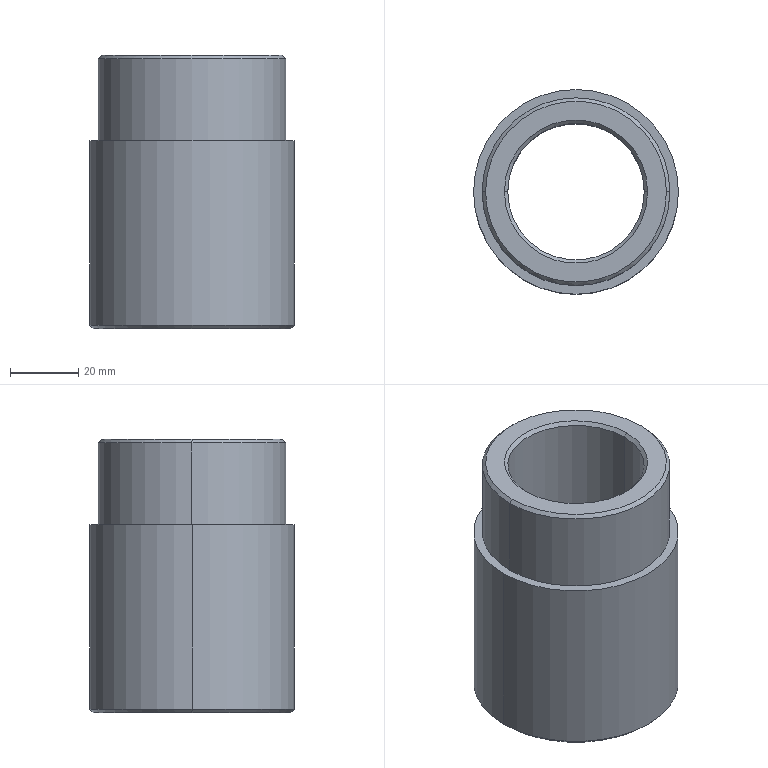Part | STEP file | Bac truot | 1 solid | 17 faces | box 60 x 60 x 80 mm | volume 114067 mm3 | cone 8 | cylinder 6 | plane 3 | commonest cylinder face diameters 40 x2 55 x2 60 x2
STEP:
#1=CARTESIAN_POINT('',(0.,0.,0.));
#2=DIRECTION('',(0.,0.,1.));
#3=DIRECTION('',(1.,0.,0.));
#4=AXIS2_PLACEMENT_3D('',#1,#2,#3);
#5=CARTESIAN_POINT('',(20.,0.,39.));
#6=VERTEX_POINT('',#5);
#7=CARTESIAN_POINT('',(21.,0.,40.));
#8=VERTEX_POINT('',#7);
#9=CARTESIAN_POINT('',(20.,0.,39.));
#10=DIRECTION('',(0.7071,0.,0.7071));
#11=VECTOR('',#10,1.);
#12=LINE('',#9,#11);
#13=CARTESIAN_POINT('',(0.,0.,39.));
#14=DIRECTION('',(0.,0.,1.));
#15=DIRECTION('',(1.,0.,0.));
#16=AXIS2_PLACEMENT_3D('',#13,#14,#15);
#17=CONICAL_SURFACE('',#16,20.,0.7854);
#18=CARTESIAN_POINT('',(6.283,0.));
#19=DIRECTION('',(0.,1.));
#20=VECTOR('',#19,1.);
#21=LINE('',#18,#20);
#22=(GEOMETRIC_REPRESENTATION_CONTEXT(2)PARAMETRIC_REPRESENTATION_CONTEXT()REPRESENTATION_CONTEXT('',''));
#23=DEFINITIONAL_REPRESENTATION('',(#21),#22);
#24=PCURVE('',#17,#23);
#25=CARTESIAN_POINT('',(0.,0.,39.));
#26=DIRECTION('',(0.,0.,1.));
#27=DIRECTION('',(1.,0.,0.));
#28=AXIS2_PLACEMENT_3D('',#25,#26,#27);
#29=CONICAL_SURFACE('',#28,20.,0.7854);
#30=CARTESIAN_POINT('',(0.,0.));
#31=DIRECTION('',(0.,1.));
#32=VECTOR('',#31,1.);
#33=LINE('',#30,#32);
#34=(GEOMETRIC_REPRESENTATION_CONTEXT(2)PARAMETRIC_REPRESENTATION_CONTEXT()REPRESENTATION_CONTEXT('',''));
#35=DEFINITIONAL_REPRESENTATION('',(#33),#34);
#36=PCURVE('',#29,#35);
#37=SURFACE_CURVE('',#12,(#24,#36),.PCURVE_S1.);
#38=EDGE_CURVE('',#6,#8,#37,.T.);
#39=ORIENTED_EDGE('',*,*,#38,.T.);
#40=CARTESIAN_POINT('',(-21.,0.,40.));
#41=VERTEX_POINT('',#40);
#42=CARTESIAN_POINT('',(0.,0.,40.));
#43=DIRECTION('',(0.,0.,-1.));
#44=DIRECTION('',(1.,0.,0.));
#45=AXIS2_PLACEMENT_3D('',#42,#43,#44);
#46=CIRCLE('',#45,21.);
#47=CARTESIAN_POINT('',(6.283,1.));
#48=DIRECTION('',(-1.,0.));
#49=VECTOR('',#48,1.);
#50=LINE('',#47,#49);
#51=(GEOMETRIC_REPRESENTATION_CONTEXT(2)PARAMETRIC_REPRESENTATION_CONTEXT()REPRESENTATION_CONTEXT('',''));
#52=DEFINITIONAL_REPRESENTATION('',(#50),#51);
#53=PCURVE('',#17,#52);
#54=CARTESIAN_POINT('',(0.,0.,40.));
#55=DIRECTION('',(0.,0.,1.));
#56=DIRECTION('',(1.,0.,0.));
#57=AXIS2_PLACEMENT_3D('',#54,#55,#56);
#58=PLANE('',#57);
#59=CARTESIAN_POINT('',(21.,0.));
#60=CARTESIAN_POINT('',(21.,-36.373));
#61=CARTESIAN_POINT('',(-10.5,-18.187));
#62=CARTESIAN_POINT('',(-42.,0.));
#63=CARTESIAN_POINT('',(-10.5,18.187));
#64=CARTESIAN_POINT('',(21.,36.373));
#65=CARTESIAN_POINT('',(21.,0.));
#66=(BOUNDED_CURVE()B_SPLINE_CURVE(2,(#59,#60,#61,#62,#63,#64,#65),.UNSPECIFIED.,.T.,.F.)B_SPLINE_CURVE_WITH_KNOTS((1,2,2,2,2,1),(-2.094,0.,2.094,4.189,6.283,8.378),.UNSPECIFIED.)CURVE()GEOMETRIC_REPRESENTATION_ITEM()RATIONAL_B_SPLINE_CURVE((1.,0.5,1.,0.5,1.,0.5,1.))REPRESENTATION_ITEM(''));
#67=(GEOMETRIC_REPRESENTATION_CONTEXT(2)PARAMETRIC_REPRESENTATION_CONTEXT()REPRESENTATION_CONTEXT('',''));
#68=DEFINITIONAL_REPRESENTATION('',(#66),#67);
#69=PCURVE('',#58,#68);
#70=SURFACE_CURVE('',#46,(#53,#69),.PCURVE_S1.);
#71=EDGE_CURVE('',#8,#41,#70,.T.);
#72=ORIENTED_EDGE('',*,*,#71,.T.);
#73=CARTESIAN_POINT('',(-20.,0.,39.));
#74=VERTEX_POINT('',#73);
#75=CARTESIAN_POINT('',(-20.,0.,39.));
#76=DIRECTION('',(-0.7071,0.,0.7071));
#77=VECTOR('',#76,1.);
#78=LINE('',#75,#77);
#79=CARTESIAN_POINT('',(3.142,0.));
#80=DIRECTION('',(0.,1.));
#81=VECTOR('',#80,1.);
#82=LINE('',#79,#81);
#83=(GEOMETRIC_REPRESENTATION_CONTEXT(2)PARAMETRIC_REPRESENTATION_CONTEXT()REPRESENTATION_CONTEXT('',''));
#84=DEFINITIONAL_REPRESENTATION('',(#82),#83);
#85=PCURVE('',#17,#84);
#86=CARTESIAN_POINT('',(3.142,0.));
#87=DIRECTION('',(0.,1.));
#88=VECTOR('',#87,1.);
#89=LINE('',#86,#88);
#90=(GEOMETRIC_REPRESENTATION_CONTEXT(2)PARAMETRIC_REPRESENTATION_CONTEXT()REPRESENTATION_CONTEXT('',''));
#91=DEFINITIONAL_REPRESENTATION('',(#89),#90);
#92=PCURVE('',#29,#91);
#93=SURFACE_CURVE('',#78,(#85,#92),.PCURVE_S1.);
#94=EDGE_CURVE('',#74,#41,#93,.T.);
#95=ORIENTED_EDGE('',*,*,#94,.F.);
#96=CARTESIAN_POINT('',(0.,0.,39.));
#97=DIRECTION('',(0.,0.,1.));
#98=DIRECTION('',(1.,0.,0.));
#99=AXIS2_PLACEMENT_3D('',#96,#97,#98);
#100=CIRCLE('',#99,20.);
#101=CARTESIAN_POINT('',(0.,0.));
#102=DIRECTION('',(1.,0.));
#103=VECTOR('',#102,1.);
#104=LINE('',#101,#103);
#105=(GEOMETRIC_REPRESENTATION_CONTEXT(2)PARAMETRIC_REPRESENTATION_CONTEXT()REPRESENTATION_CONTEXT('',''));
#106=DEFINITIONAL_REPRESENTATION('',(#104),#105);
#107=PCURVE('',#17,#106);
#108=CARTESIAN_POINT('',(0.,0.,40.));
#109=DIRECTION('',(0.,0.,-1.));
#110=DIRECTION('',(-1.,0.,0.));
#111=AXIS2_PLACEMENT_3D('',#108,#109,#110);
#112=CYLINDRICAL_SURFACE('',#111,20.);
#113=CARTESIAN_POINT('',(9.425,1.));
#114=DIRECTION('',(-1.,0.));
#115=VECTOR('',#114,1.);
#116=LINE('',#113,#115);
#117=(GEOMETRIC_REPRESENTATION_CONTEXT(2)PARAMETRIC_REPRESENTATION_CONTEXT()REPRESENTATION_CONTEXT('',''));
#118=DEFINITIONAL_REPRESENTATION('',(#116),#117);
#119=PCURVE('',#112,#118);
#120=SURFACE_CURVE('',#100,(#107,#119),.PCURVE_S1.);
#121=EDGE_CURVE('',#74,#6,#120,.T.);
#122=ORIENTED_EDGE('',*,*,#121,.T.);
#123=EDGE_LOOP('',(#39,#72,#95,#122));
#124=FACE_BOUND('',#123,.F.);
#125=ADVANCED_FACE('',(#124),#17,.F.);
#126=CARTESIAN_POINT('',(26.5,0.,40.));
#127=VERTEX_POINT('',#126);
#128=CARTESIAN_POINT('',(-26.5,0.,40.));
#129=VERTEX_POINT('',#128);
#130=CARTESIAN_POINT('',(0.,0.,40.));
#131=DIRECTION('',(0.,0.,1.));
#132=DIRECTION('',(1.,0.,0.));
#133=AXIS2_PLACEMENT_3D('',#130,#131,#132);
#134=CIRCLE('',#133,26.5);
#135=CARTESIAN_POINT('',(0.,0.,40.));
#136=DIRECTION('',(0.,0.,-1.));
#137=DIRECTION('',(-1.,0.,0.));
#138=AXIS2_PLACEMENT_3D('',#135,#136,#137);
#139=CONICAL_SURFACE('',#138,26.5,0.7854);
#140=CARTESIAN_POINT('',(3.142,0.));
#141=DIRECTION('',(-1.,0.));
#142=VECTOR('',#141,1.);
#143=LINE('',#140,#142);
#144=(GEOMETRIC_REPRESENTATION_CONTEXT(2)PARAMETRIC_REPRESENTATION_CONTEXT()REPRESENTATION_CONTEXT('',''));
#145=DEFINITIONAL_REPRESENTATION('',(#143),#144);
#146=PCURVE('',#139,#145);
#147=CARTESIAN_POINT('',(0.,0.));
#148=DIRECTION('',(1.,0.));
#149=AXIS2_PLACEMENT_2D('',#147,#148);
#150=CIRCLE('',#149,26.5);
#151=(GEOMETRIC_REPRESENTATION_CONTEXT(2)PARAMETRIC_REPRESENTATION_CONTEXT()REPRESENTATION_CONTEXT('',''));
#152=DEFINITIONAL_REPRESENTATION('',(#150),#151);
#153=PCURVE('',#58,#152);
#154=SURFACE_CURVE('',#134,(#146,#153),.PCURVE_S1.);
#155=EDGE_CURVE('',#127,#129,#154,.T.);
#156=ORIENTED_EDGE('',*,*,#155,.F.);
#157=CARTESIAN_POINT('',(27.5,0.,39.));
#158=VERTEX_POINT('',#157);
#159=CARTESIAN_POINT('',(26.5,0.,40.));
#160=DIRECTION('',(0.7071,0.,-0.7071));
#161=VECTOR('',#160,1.);
#162=LINE('',#159,#161);
#163=CARTESIAN_POINT('',(3.142,0.));
#164=DIRECTION('',(0.,1.));
#165=VECTOR('',#164,1.);
#166=LINE('',#163,#165);
#167=(GEOMETRIC_REPRESENTATION_CONTEXT(2)PARAMETRIC_REPRESENTATION_CONTEXT()REPRESENTATION_CONTEXT('',''));
#168=DEFINITIONAL_REPRESENTATION('',(#166),#167);
#169=PCURVE('',#139,#168);
#170=CARTESIAN_POINT('',(0.,0.,40.));
#171=DIRECTION('',(0.,0.,-1.));
#172=DIRECTION('',(-1.,0.,0.));
#173=AXIS2_PLACEMENT_3D('',#170,#171,#172);
#174=CONICAL_SURFACE('',#173,26.5,0.7854);
#175=CARTESIAN_POINT('',(3.142,0.));
#176=DIRECTION('',(0.,1.));
#177=VECTOR('',#176,1.);
#178=LINE('',#175,#177);
#179=(GEOMETRIC_REPRESENTATION_CONTEXT(2)PARAMETRIC_REPRESENTATION_CONTEXT()REPRESENTATION_CONTEXT('',''));
#180=DEFINITIONAL_REPRESENTATION('',(#178),#179);
#181=PCURVE('',#174,#180);
#182=SURFACE_CURVE('',#162,(#169,#181),.PCURVE_S1.);
#183=EDGE_CURVE('',#127,#158,#182,.T.);
#184=ORIENTED_EDGE('',*,*,#183,.T.);
#185=CARTESIAN_POINT('',(-27.5,0.,39.));
#186=VERTEX_POINT('',#185);
#187=CARTESIAN_POINT('',(0.,0.,39.));
#188=DIRECTION('',(0.,0.,-1.));
#189=DIRECTION('',(1.,0.,0.));
#190=AXIS2_PLACEMENT_3D('',#187,#188,#189);
#191=CIRCLE('',#190,27.5);
#192=CARTESIAN_POINT('',(-3.142,1.));
#193=DIRECTION('',(1.,0.));
#194=VECTOR('',#193,1.);
#195=LINE('',#192,#194);
#196=(GEOMETRIC_REPRESENTATION_CONTEXT(2)PARAMETRIC_REPRESENTATION_CONTEXT()REPRESENTATION_CONTEXT('',''));
#197=DEFINITIONAL_REPRESENTATION('',(#195),#196);
#198=PCURVE('',#139,#197);
#199=CARTESIAN_POINT('',(0.,0.,15.));
#200=DIRECTION('',(0.,0.,1.));
#201=DIRECTION('',(1.,0.,0.));
#202=AXIS2_PLACEMENT_3D('',#199,#200,#201);
#203=CYLINDRICAL_SURFACE('',#202,27.5);
#204=CARTESIAN_POINT('',(6.283,24.));
#205=DIRECTION('',(-1.,0.));
#206=VECTOR('',#205,1.);
#207=LINE('',#204,#206);
#208=(GEOMETRIC_REPRESENTATION_CONTEXT(2)PARAMETRIC_REPRESENTATION_CONTEXT()REPRESENTATION_CONTEXT('',''));
#209=DEFINITIONAL_REPRESENTATION('',(#207),#208);
#210=PCURVE('',#203,#209);
#211=SURFACE_CURVE('',#191,(#198,#210),.PCURVE_S1.);
#212=EDGE_CURVE('',#186,#158,#211,.T.);
#213=ORIENTED_EDGE('',*,*,#212,.F.);
#214=CARTESIAN_POINT('',(-26.5,0.,40.));
#215=DIRECTION('',(-0.7071,0.,-0.7071));
#216=VECTOR('',#215,1.);
#217=LINE('',#214,#216);
#218=CARTESIAN_POINT('',(0.,0.));
#219=DIRECTION('',(0.,1.));
#220=VECTOR('',#219,1.);
#221=LINE('',#218,#220);
#222=(GEOMETRIC_REPRESENTATION_CONTEXT(2)PARAMETRIC_REPRESENTATION_CONTEXT()REPRESENTATION_CONTEXT('',''));
#223=DEFINITIONAL_REPRESENTATION('',(#221),#222);
#224=PCURVE('',#139,#223);
#225=CARTESIAN_POINT('',(6.283,0.));
#226=DIRECTION('',(0.,1.));
#227=VECTOR('',#226,1.);
#228=LINE('',#225,#227);
#229=(GEOMETRIC_REPRESENTATION_CONTEXT(2)PARAMETRIC_REPRESENTATION_CONTEXT()REPRESENTATION_CONTEXT('',''));
#230=DEFINITIONAL_REPRESENTATION('',(#228),#229);
#231=PCURVE('',#174,#230);
#232=SURFACE_CURVE('',#217,(#224,#231),.PCURVE_S1.);
#233=EDGE_CURVE('',#129,#186,#232,.T.);
#234=ORIENTED_EDGE('',*,*,#233,.F.);
#235=EDGE_LOOP('',(#156,#184,#213,#234));
#236=FACE_BOUND('',#235,.T.);
#237=ADVANCED_FACE('',(#236),#139,.T.);
#238=CARTESIAN_POINT('',(-29.,0.,-40.));
#239=VERTEX_POINT('',#238);
#240=CARTESIAN_POINT('',(29.,0.,-40.));
#241=VERTEX_POINT('',#240);
#242=CARTESIAN_POINT('',(0.,0.,-40.));
#243=DIRECTION('',(0.,0.,-1.));
#244=DIRECTION('',(1.,0.,0.));
#245=AXIS2_PLACEMENT_3D('',#242,#243,#244);
#246=CIRCLE('',#245,29.);
#247=CARTESIAN_POINT('',(0.,0.,-39.));
#248=DIRECTION('',(0.,0.,1.));
#249=DIRECTION('',(1.,0.,0.));
#250=AXIS2_PLACEMENT_3D('',#247,#248,#249);
#251=CONICAL_SURFACE('',#250,30.,0.7854);
#252=CARTESIAN_POINT('',(6.283,-1.));
#253=DIRECTION('',(-1.,0.));
#254=VECTOR('',#253,1.);
#255=LINE('',#252,#254);
#256=(GEOMETRIC_REPRESENTATION_CONTEXT(2)PARAMETRIC_REPRESENTATION_CONTEXT()REPRESENTATION_CONTEXT('',''));
#257=DEFINITIONAL_REPRESENTATION('',(#255),#256);
#258=PCURVE('',#251,#257);
#259=CARTESIAN_POINT('',(0.,0.,-40.));
#260=DIRECTION('',(0.,0.,1.));
#261=DIRECTION('',(1.,0.,0.));
#262=AXIS2_PLACEMENT_3D('',#259,#260,#261);
#263=PLANE('',#262);
#264=CARTESIAN_POINT('',(29.,0.));
#265=CARTESIAN_POINT('',(29.,-50.229));
#266=CARTESIAN_POINT('',(-14.5,-25.115));
#267=CARTESIAN_POINT('',(-58.,0.));
#268=CARTESIAN_POINT('',(-14.5,25.115));
#269=CARTESIAN_POINT('',(29.,50.229));
#270=CARTESIAN_POINT('',(29.,0.));
#271=(BOUNDED_CURVE()B_SPLINE_CURVE(2,(#264,#265,#266,#267,#268,#269,#270),.UNSPECIFIED.,.T.,.F.)B_SPLINE_CURVE_WITH_KNOTS((1,2,2,2,2,1),(-2.094,0.,2.094,4.189,6.283,8.378),.UNSPECIFIED.)CURVE()GEOMETRIC_REPRESENTATION_ITEM()RATIONAL_B_SPLINE_CURVE((1.,0.5,1.,0.5,1.,0.5,1.))REPRESENTATION_ITEM(''));
#272=(GEOMETRIC_REPRESENTATION_CONTEXT(2)PARAMETRIC_REPRESENTATION_CONTEXT()REPRESENTATION_CONTEXT('',''));
#273=DEFINITIONAL_REPRESENTATION('',(#271),#272);
#274=PCURVE('',#263,#273);
#275=SURFACE_CURVE('',#246,(#258,#274),.PCURVE_S1.);
#276=EDGE_CURVE('',#239,#241,#275,.T.);
#277=ORIENTED_EDGE('',*,*,#276,.F.);
#278=CARTESIAN_POINT('',(-30.,0.,-39.));
#279=VERTEX_POINT('',#278);
#280=CARTESIAN_POINT('',(-30.,0.,-39.));
#281=DIRECTION('',(-0.7071,0.,0.7071));
#282=VECTOR('',#281,1.);
#283=LINE('',#280,#282);
#284=CARTESIAN_POINT('',(3.142,0.));
#285=DIRECTION('',(0.,1.));
#286=VECTOR('',#285,1.);
#287=LINE('',#284,#286);
#288=(GEOMETRIC_REPRESENTATION_CONTEXT(2)PARAMETRIC_REPRESENTATION_CONTEXT()REPRESENTATION_CONTEXT('',''));
#289=DEFINITIONAL_REPRESENTATION('',(#287),#288);
#290=PCURVE('',#251,#289);
#291=CARTESIAN_POINT('',(0.,0.,-39.));
#292=DIRECTION('',(0.,0.,1.));
#293=DIRECTION('',(1.,0.,0.));
#294=AXIS2_PLACEMENT_3D('',#291,#292,#293);
#295=CONICAL_SURFACE('',#294,30.,0.7854);
#296=CARTESIAN_POINT('',(3.142,0.));
#297=DIRECTION('',(0.,1.));
#298=VECTOR('',#297,1.);
#299=LINE('',#296,#298);
#300=(GEOMETRIC_REPRESENTATION_CONTEXT(2)PARAMETRIC_REPRESENTATION_CONTEXT()REPRESENTATION_CONTEXT('',''));
#301=DEFINITIONAL_REPRESENTATION('',(#299),#300);
#302=PCURVE('',#295,#301);
#303=SURFACE_CURVE('',#283,(#290,#302),.PCURVE_S1.);
#304=EDGE_CURVE('',#239,#279,#303,.T.);
#305=ORIENTED_EDGE('',*,*,#304,.T.);
#306=CARTESIAN_POINT('',(30.,0.,-39.));
#307=VERTEX_POINT('',#306);
#308=CARTESIAN_POINT('',(0.,0.,-39.));
#309=DIRECTION('',(0.,0.,1.));
#310=DIRECTION('',(1.,0.,0.));
#311=AXIS2_PLACEMENT_3D('',#308,#309,#310);
#312=CIRCLE('',#311,30.);
#313=CARTESIAN_POINT('',(0.,0.));
#314=DIRECTION('',(1.,0.));
#315=VECTOR('',#314,1.);
#316=LINE('',#313,#315);
#317=(GEOMETRIC_REPRESENTATION_CONTEXT(2)PARAMETRIC_REPRESENTATION_CONTEXT()REPRESENTATION_CONTEXT('',''));
#318=DEFINITIONAL_REPRESENTATION('',(#316),#317);
#319=PCURVE('',#251,#318);
#320=CARTESIAN_POINT('',(0.,0.,40.));
#321=DIRECTION('',(0.,0.,-1.));
#322=DIRECTION('',(-1.,0.,0.));
#323=AXIS2_PLACEMENT_3D('',#320,#321,#322);
#324=CYLINDRICAL_SURFACE('',#323,30.);
#325=CARTESIAN_POINT('',(3.142,79.));
#326=DIRECTION('',(-1.,0.));
#327=VECTOR('',#326,1.);
#328=LINE('',#325,#327);
#329=(GEOMETRIC_REPRESENTATION_CONTEXT(2)PARAMETRIC_REPRESENTATION_CONTEXT()REPRESENTATION_CONTEXT('',''));
#330=DEFINITIONAL_REPRESENTATION('',(#328),#329);
#331=PCURVE('',#324,#330);
#332=SURFACE_CURVE('',#312,(#319,#331),.PCURVE_S1.);
#333=EDGE_CURVE('',#307,#279,#332,.T.);
#334=ORIENTED_EDGE('',*,*,#333,.F.);
#335=CARTESIAN_POINT('',(30.,0.,-39.));
#336=DIRECTION('',(0.7071,0.,0.7071));
#337=VECTOR('',#336,1.);
#338=LINE('',#335,#337);
#339=CARTESIAN_POINT('',(0.,0.));
#340=DIRECTION('',(0.,1.));
#341=VECTOR('',#340,1.);
#342=LINE('',#339,#341);
#343=(GEOMETRIC_REPRESENTATION_CONTEXT(2)PARAMETRIC_REPRESENTATION_CONTEXT()REPRESENTATION_CONTEXT('',''));
#344=DEFINITIONAL_REPRESENTATION('',(#342),#343);
#345=PCURVE('',#251,#344);
#346=CARTESIAN_POINT('',(6.283,0.));
#347=DIRECTION('',(0.,1.));
#348=VECTOR('',#347,1.);
#349=LINE('',#346,#348);
#350=(GEOMETRIC_REPRESENTATION_CONTEXT(2)PARAMETRIC_REPRESENTATION_CONTEXT()REPRESENTATION_CONTEXT('',''));
#351=DEFINITIONAL_REPRESENTATION('',(#349),#350);
#352=PCURVE('',#295,#351);
#353=SURFACE_CURVE('',#338,(#345,#352),.PCURVE_S1.);
#354=EDGE_CURVE('',#241,#307,#353,.T.);
#355=ORIENTED_EDGE('',*,*,#354,.F.);
#356=EDGE_LOOP('',(#277,#305,#334,#355));
#357=FACE_BOUND('',#356,.T.);
#358=ADVANCED_FACE('',(#357),#251,.T.);
#359=CARTESIAN_POINT('',(-20.,0.,-39.));
#360=VERTEX_POINT('',#359);
#361=CARTESIAN_POINT('',(-21.,0.,-40.));
#362=VERTEX_POINT('',#361);
#363=CARTESIAN_POINT('',(-21.,0.,-40.));
#364=DIRECTION('',(-0.7071,0.,-0.7071));
#365=VECTOR('',#364,1.);
#366=LINE('',#363,#365);
#367=CARTESIAN_POINT('',(0.,0.,-40.));
#368=DIRECTION('',(0.,0.,-1.));
#369=DIRECTION('',(-1.,0.,0.));
#370=AXIS2_PLACEMENT_3D('',#367,#368,#369);
#371=CONICAL_SURFACE('',#370,21.,0.7854);
#372=CARTESIAN_POINT('',(6.283,0.));
#373=DIRECTION('',(0.,1.));
#374=VECTOR('',#373,1.);
#375=LINE('',#372,#374);
#376=(GEOMETRIC_REPRESENTATION_CONTEXT(2)PARAMETRIC_REPRESENTATION_CONTEXT()REPRESENTATION_CONTEXT('',''));
#377=DEFINITIONAL_REPRESENTATION('',(#375),#376);
#378=PCURVE('',#371,#377);
#379=CARTESIAN_POINT('',(0.,0.,-40.));
#380=DIRECTION('',(0.,0.,-1.));
#381=DIRECTION('',(-1.,0.,0.));
#382=AXIS2_PLACEMENT_3D('',#379,#380,#381);
#383=CONICAL_SURFACE('',#382,21.,0.7854);
#384=CARTESIAN_POINT('',(0.,0.));
#385=DIRECTION('',(0.,1.));
#386=VECTOR('',#385,1.);
#387=LINE('',#384,#386);
#388=(GEOMETRIC_REPRESENTATION_CONTEXT(2)PARAMETRIC_REPRESENTATION_CONTEXT()REPRESENTATION_CONTEXT('',''));
#389=DEFINITIONAL_REPRESENTATION('',(#387),#388);
#390=PCURVE('',#383,#389);
#391=SURFACE_CURVE('',#366,(#378,#390),.PCURVE_S1.);
#392=EDGE_CURVE('',#360,#362,#391,.T.);
#393=ORIENTED_EDGE('',*,*,#392,.T.);
#394=CARTESIAN_POINT('',(21.,0.,-40.));
#395=VERTEX_POINT('',#394);
#396=CARTESIAN_POINT('',(0.,0.,-40.));
#397=DIRECTION('',(0.,0.,1.));
#398=DIRECTION('',(1.,0.,0.));
#399=AXIS2_PLACEMENT_3D('',#396,#397,#398);
#400=CIRCLE('',#399,21.);
#401=CARTESIAN_POINT('',(9.425,0.));
#402=DIRECTION('',(-1.,0.));
#403=VECTOR('',#402,1.);
#404=LINE('',#401,#403);
#405=(GEOMETRIC_REPRESENTATION_CONTEXT(2)PARAMETRIC_REPRESENTATION_CONTEXT()REPRESENTATION_CONTEXT('',''));
#406=DEFINITIONAL_REPRESENTATION('',(#404),#405);
#407=PCURVE('',#371,#406);
#408=CARTESIAN_POINT('',(0.,0.));
#409=DIRECTION('',(1.,0.));
#410=AXIS2_PLACEMENT_2D('',#408,#409);
#411=CIRCLE('',#410,21.);
#412=(GEOMETRIC_REPRESENTATION_CONTEXT(2)PARAMETRIC_REPRESENTATION_CONTEXT()REPRESENTATION_CONTEXT('',''));
#413=DEFINITIONAL_REPRESENTATION('',(#411),#412);
#414=PCURVE('',#263,#413);
#415=SURFACE_CURVE('',#400,(#407,#414),.PCURVE_S1.);
#416=EDGE_CURVE('',#362,#395,#415,.T.);
#417=ORIENTED_EDGE('',*,*,#416,.T.);
#418=CARTESIAN_POINT('',(20.,0.,-39.));
#419=VERTEX_POINT('',#418);
#420=CARTESIAN_POINT('',(21.,0.,-40.));
#421=DIRECTION('',(0.7071,0.,-0.7071));
#422=VECTOR('',#421,1.);
#423=LINE('',#420,#422);
#424=CARTESIAN_POINT('',(3.142,0.));
#425=DIRECTION('',(0.,1.));
#426=VECTOR('',#425,1.);
#427=LINE('',#424,#426);
#428=(GEOMETRIC_REPRESENTATION_CONTEXT(2)PARAMETRIC_REPRESENTATION_CONTEXT()REPRESENTATION_CONTEXT('',''));
#429=DEFINITIONAL_REPRESENTATION('',(#427),#428);
#430=PCURVE('',#371,#429);
#431=CARTESIAN_POINT('',(3.142,0.));
#432=DIRECTION('',(0.,1.));
#433=VECTOR('',#432,1.);
#434=LINE('',#431,#433);
#435=(GEOMETRIC_REPRESENTATION_CONTEXT(2)PARAMETRIC_REPRESENTATION_CONTEXT()REPRESENTATION_CONTEXT('',''));
#436=DEFINITIONAL_REPRESENTATION('',(#434),#435);
#437=PCURVE('',#383,#436);
#438=SURFACE_CURVE('',#423,(#430,#437),.PCURVE_S1.);
#439=EDGE_CURVE('',#419,#395,#438,.T.);
#440=ORIENTED_EDGE('',*,*,#439,.F.);
#441=CARTESIAN_POINT('',(0.,0.,-39.));
#442=DIRECTION('',(0.,0.,-1.));
#443=DIRECTION('',(1.,0.,0.));
#444=AXIS2_PLACEMENT_3D('',#441,#442,#443);
#445=CIRCLE('',#444,20.);
#446=CARTESIAN_POINT('',(3.142,-1.));
#447=DIRECTION('',(1.,0.));
#448=VECTOR('',#447,1.);
#449=LINE('',#446,#448);
#450=(GEOMETRIC_REPRESENTATION_CONTEXT(2)PARAMETRIC_REPRESENTATION_CONTEXT()REPRESENTATION_CONTEXT('',''));
#451=DEFINITIONAL_REPRESENTATION('',(#449),#450);
#452=PCURVE('',#371,#451);
#453=CARTESIAN_POINT('',(3.142,79.));
#454=DIRECTION('',(1.,0.));
#455=VECTOR('',#454,1.);
#456=LINE('',#453,#455);
#457=(GEOMETRIC_REPRESENTATION_CONTEXT(2)PARAMETRIC_REPRESENTATION_CONTEXT()REPRESENTATION_CONTEXT('',''));
#458=DEFINITIONAL_REPRESENTATION('',(#456),#457);
#459=PCURVE('',#112,#458);
#460=SURFACE_CURVE('',#445,(#452,#459),.PCURVE_S1.);
#461=EDGE_CURVE('',#419,#360,#460,.T.);
#462=ORIENTED_EDGE('',*,*,#461,.T.);
#463=EDGE_LOOP('',(#393,#417,#440,#462));
#464=FACE_BOUND('',#463,.F.);
#465=ADVANCED_FACE('',(#464),#371,.F.);
#466=CARTESIAN_POINT('',(27.5,0.,15.));
#467=VERTEX_POINT('',#466);
#468=CARTESIAN_POINT('',(-27.5,0.,15.));
#469=VERTEX_POINT('',#468);
#470=CARTESIAN_POINT('',(0.,0.,15.));
#471=DIRECTION('',(0.,0.,1.));
#472=DIRECTION('',(1.,0.,0.));
#473=AXIS2_PLACEMENT_3D('',#470,#471,#472);
#474=CIRCLE('',#473,27.5);
#475=CARTESIAN_POINT('',(0.,0.));
#476=DIRECTION('',(1.,0.));
#477=VECTOR('',#476,1.);
#478=LINE('',#475,#477);
#479=(GEOMETRIC_REPRESENTATION_CONTEXT(2)PARAMETRIC_REPRESENTATION_CONTEXT()REPRESENTATION_CONTEXT('',''));
#480=DEFINITIONAL_REPRESENTATION('',(#478),#479);
#481=PCURVE('',#203,#480);
#482=CARTESIAN_POINT('',(0.,0.,15.));
#483=DIRECTION('',(0.,0.,1.));
#484=DIRECTION('',(1.,0.,0.));
#485=AXIS2_PLACEMENT_3D('',#482,#483,#484);
#486=PLANE('',#485);
#487=CARTESIAN_POINT('',(0.,0.));
#488=DIRECTION('',(1.,0.));
#489=AXIS2_PLACEMENT_2D('',#487,#488);
#490=CIRCLE('',#489,27.5);
#491=(GEOMETRIC_REPRESENTATION_CONTEXT(2)PARAMETRIC_REPRESENTATION_CONTEXT()REPRESENTATION_CONTEXT('',''));
#492=DEFINITIONAL_REPRESENTATION('',(#490),#491);
#493=PCURVE('',#486,#492);
#494=SURFACE_CURVE('',#474,(#481,#493),.PCURVE_S1.);
#495=EDGE_CURVE('',#467,#469,#494,.T.);
#496=ORIENTED_EDGE('',*,*,#495,.T.);
#497=CARTESIAN_POINT('',(-27.5,0.,15.));
#498=DIRECTION('',(0.,0.,1.));
#499=VECTOR('',#498,1.);
#500=LINE('',#497,#499);
#501=CARTESIAN_POINT('',(3.142,0.));
#502=DIRECTION('',(0.,1.));
#503=VECTOR('',#502,1.);
#504=LINE('',#501,#503);
#505=(GEOMETRIC_REPRESENTATION_CONTEXT(2)PARAMETRIC_REPRESENTATION_CONTEXT()REPRESENTATION_CONTEXT('',''));
#506=DEFINITIONAL_REPRESENTATION('',(#504),#505);
#507=PCURVE('',#203,#506);
#508=CARTESIAN_POINT('',(0.,0.,15.));
#509=DIRECTION('',(0.,0.,1.));
#510=DIRECTION('',(1.,0.,0.));
#511=AXIS2_PLACEMENT_3D('',#508,#509,#510);
#512=CYLINDRICAL_SURFACE('',#511,27.5);
#513=CARTESIAN_POINT('',(3.142,0.));
#514=DIRECTION('',(0.,1.));
#515=VECTOR('',#514,1.);
#516=LINE('',#513,#515);
#517=(GEOMETRIC_REPRESENTATION_CONTEXT(2)PARAMETRIC_REPRESENTATION_CONTEXT()REPRESENTATION_CONTEXT('',''));
#518=DEFINITIONAL_REPRESENTATION('',(#516),#517);
#519=PCURVE('',#512,#518);
#520=SURFACE_CURVE('',#500,(#507,#519),.PCURVE_S1.);
#521=EDGE_CURVE('',#469,#186,#520,.T.);
#522=ORIENTED_EDGE('',*,*,#521,.T.);
#523=ORIENTED_EDGE('',*,*,#212,.T.);
#524=CARTESIAN_POINT('',(27.5,0.,15.));
#525=DIRECTION('',(0.,0.,1.));
#526=VECTOR('',#525,1.);
#527=LINE('',#524,#526);
#528=CARTESIAN_POINT('',(0.,0.));
#529=DIRECTION('',(0.,1.));
#530=VECTOR('',#529,1.);
#531=LINE('',#528,#530);
#532=(GEOMETRIC_REPRESENTATION_CONTEXT(2)PARAMETRIC_REPRESENTATION_CONTEXT()REPRESENTATION_CONTEXT('',''));
#533=DEFINITIONAL_REPRESENTATION('',(#531),#532);
#534=PCURVE('',#203,#533);
#535=CARTESIAN_POINT('',(6.283,0.));
#536=DIRECTION('',(0.,1.));
#537=VECTOR('',#536,1.);
#538=LINE('',#535,#537);
#539=(GEOMETRIC_REPRESENTATION_CONTEXT(2)PARAMETRIC_REPRESENTATION_CONTEXT()REPRESENTATION_CONTEXT('',''));
#540=DEFINITIONAL_REPRESENTATION('',(#538),#539);
#541=PCURVE('',#512,#540);
#542=SURFACE_CURVE('',#527,(#534,#541),.PCURVE_S1.);
#543=EDGE_CURVE('',#467,#158,#542,.T.);
#544=ORIENTED_EDGE('',*,*,#543,.F.);
#545=EDGE_LOOP('',(#496,#522,#523,#544));
#546=FACE_BOUND('',#545,.T.);
#547=ADVANCED_FACE('',(#546),#203,.T.);
#548=CARTESIAN_POINT('',(-20.,0.,40.));
#549=DIRECTION('',(0.,0.,-1.));
#550=VECTOR('',#549,1.);
#551=LINE('',#548,#550);
#552=CARTESIAN_POINT('',(6.283,0.));
#553=DIRECTION('',(0.,1.));
#554=VECTOR('',#553,1.);
#555=LINE('',#552,#554);
#556=(GEOMETRIC_REPRESENTATION_CONTEXT(2)PARAMETRIC_REPRESENTATION_CONTEXT()REPRESENTATION_CONTEXT('',''));
#557=DEFINITIONAL_REPRESENTATION('',(#555),#556);
#558=PCURVE('',#112,#557);
#559=CARTESIAN_POINT('',(0.,0.,40.));
#560=DIRECTION('',(0.,0.,-1.));
#561=DIRECTION('',(-1.,0.,0.));
#562=AXIS2_PLACEMENT_3D('',#559,#560,#561);
#563=CYLINDRICAL_SURFACE('',#562,20.);
#564=CARTESIAN_POINT('',(0.,0.));
#565=DIRECTION('',(0.,1.));
#566=VECTOR('',#565,1.);
#567=LINE('',#564,#566);
#568=(GEOMETRIC_REPRESENTATION_CONTEXT(2)PARAMETRIC_REPRESENTATION_CONTEXT()REPRESENTATION_CONTEXT('',''));
#569=DEFINITIONAL_REPRESENTATION('',(#567),#568);
#570=PCURVE('',#563,#569);
#571=SURFACE_CURVE('',#551,(#558,#570),.PCURVE_S1.);
#572=EDGE_CURVE('',#74,#360,#571,.T.);
#573=ORIENTED_EDGE('',*,*,#572,.T.);
#574=ORIENTED_EDGE('',*,*,#461,.F.);
#575=CARTESIAN_POINT('',(20.,0.,40.));
#576=DIRECTION('',(0.,0.,-1.));
#577=VECTOR('',#576,1.);
#578=LINE('',#575,#577);
#579=CARTESIAN_POINT('',(3.142,0.));
#580=DIRECTION('',(0.,1.));
#581=VECTOR('',#580,1.);
#582=LINE('',#579,#581);
#583=(GEOMETRIC_REPRESENTATION_CONTEXT(2)PARAMETRIC_REPRESENTATION_CONTEXT()REPRESENTATION_CONTEXT('',''));
#584=DEFINITIONAL_REPRESENTATION('',(#582),#583);
#585=PCURVE('',#112,#584);
#586=CARTESIAN_POINT('',(3.142,0.));
#587=DIRECTION('',(0.,1.));
#588=VECTOR('',#587,1.);
#589=LINE('',#586,#588);
#590=(GEOMETRIC_REPRESENTATION_CONTEXT(2)PARAMETRIC_REPRESENTATION_CONTEXT()REPRESENTATION_CONTEXT('',''));
#591=DEFINITIONAL_REPRESENTATION('',(#589),#590);
#592=PCURVE('',#563,#591);
#593=SURFACE_CURVE('',#578,(#585,#592),.PCURVE_S1.);
#594=EDGE_CURVE('',#6,#419,#593,.T.);
#595=ORIENTED_EDGE('',*,*,#594,.F.);
#596=ORIENTED_EDGE('',*,*,#121,.F.);
#597=EDGE_LOOP('',(#573,#574,#595,#596));
#598=FACE_BOUND('',#597,.F.);
#599=ADVANCED_FACE('',(#598),#112,.F.);
#600=CARTESIAN_POINT('',(30.,0.,15.));
#601=VERTEX_POINT('',#600);
#602=CARTESIAN_POINT('',(-30.,0.,15.));
#603=VERTEX_POINT('',#602);
#604=CARTESIAN_POINT('',(0.,0.,15.));
#605=DIRECTION('',(0.,0.,1.));
#606=DIRECTION('',(1.,0.,0.));
#607=AXIS2_PLACEMENT_3D('',#604,#605,#606);
#608=CIRCLE('',#607,30.);
#609=CARTESIAN_POINT('',(3.142,25.));
#610=DIRECTION('',(-1.,0.));
#611=VECTOR('',#610,1.);
#612=LINE('',#609,#611);
#613=(GEOMETRIC_REPRESENTATION_CONTEXT(2)PARAMETRIC_REPRESENTATION_CONTEXT()REPRESENTATION_CONTEXT('',''));
#614=DEFINITIONAL_REPRESENTATION('',(#612),#613);
#615=PCURVE('',#324,#614);
#616=CARTESIAN_POINT('',(0.,0.));
#617=DIRECTION('',(1.,0.));
#618=AXIS2_PLACEMENT_2D('',#616,#617);
#619=CIRCLE('',#618,30.);
#620=(GEOMETRIC_REPRESENTATION_CONTEXT(2)PARAMETRIC_REPRESENTATION_CONTEXT()REPRESENTATION_CONTEXT('',''));
#621=DEFINITIONAL_REPRESENTATION('',(#619),#620);
#622=PCURVE('',#486,#621);
#623=SURFACE_CURVE('',#608,(#615,#622),.PCURVE_S1.);
#624=EDGE_CURVE('',#601,#603,#623,.T.);
#625=ORIENTED_EDGE('',*,*,#624,.F.);
#626=CARTESIAN_POINT('',(30.,0.,40.));
#627=DIRECTION('',(0.,0.,-1.));
#628=VECTOR('',#627,1.);
#629=LINE('',#626,#628);
#630=CARTESIAN_POINT('',(3.142,0.));
#631=DIRECTION('',(0.,1.));
#632=VECTOR('',#631,1.);
#633=LINE('',#630,#632);
#634=(GEOMETRIC_REPRESENTATION_CONTEXT(2)PARAMETRIC_REPRESENTATION_CONTEXT()REPRESENTATION_CONTEXT('',''));
#635=DEFINITIONAL_REPRESENTATION('',(#633),#634);
#636=PCURVE('',#324,#635);
#637=CARTESIAN_POINT('',(0.,0.,40.));
#638=DIRECTION('',(0.,0.,-1.));
#639=DIRECTION('',(-1.,0.,0.));
#640=AXIS2_PLACEMENT_3D('',#637,#638,#639);
#641=CYLINDRICAL_SURFACE('',#640,30.);
#642=CARTESIAN_POINT('',(3.142,0.));
#643=DIRECTION('',(0.,1.));
#644=VECTOR('',#643,1.);
#645=LINE('',#642,#644);
#646=(GEOMETRIC_REPRESENTATION_CONTEXT(2)PARAMETRIC_REPRESENTATION_CONTEXT()REPRESENTATION_CONTEXT('',''));
#647=DEFINITIONAL_REPRESENTATION('',(#645),#646);
#648=PCURVE('',#641,#647);
#649=SURFACE_CURVE('',#629,(#636,#648),.PCURVE_S1.);
#650=EDGE_CURVE('',#601,#307,#649,.T.);
#651=ORIENTED_EDGE('',*,*,#650,.T.);
#652=ORIENTED_EDGE('',*,*,#333,.T.);
#653=CARTESIAN_POINT('',(-30.,0.,40.));
#654=DIRECTION('',(0.,0.,-1.));
#655=VECTOR('',#654,1.);
#656=LINE('',#653,#655);
#657=CARTESIAN_POINT('',(0.,0.));
#658=DIRECTION('',(0.,1.));
#659=VECTOR('',#658,1.);
#660=LINE('',#657,#659);
#661=(GEOMETRIC_REPRESENTATION_CONTEXT(2)PARAMETRIC_REPRESENTATION_CONTEXT()REPRESENTATION_CONTEXT('',''));
#662=DEFINITIONAL_REPRESENTATION('',(#660),#661);
#663=PCURVE('',#324,#662);
#664=CARTESIAN_POINT('',(6.283,0.));
#665=DIRECTION('',(0.,1.));
#666=VECTOR('',#665,1.);
#667=LINE('',#664,#666);
#668=(GEOMETRIC_REPRESENTATION_CONTEXT(2)PARAMETRIC_REPRESENTATION_CONTEXT()REPRESENTATION_CONTEXT('',''));
#669=DEFINITIONAL_REPRESENTATION('',(#667),#668);
#670=PCURVE('',#641,#669);
#671=SURFACE_CURVE('',#656,(#663,#670),.PCURVE_S1.);
#672=EDGE_CURVE('',#603,#279,#671,.T.);
#673=ORIENTED_EDGE('',*,*,#672,.F.);
#674=EDGE_LOOP('',(#625,#651,#652,#673));
#675=FACE_BOUND('',#674,.T.);
#676=ADVANCED_FACE('',(#675),#324,.T.);
#677=CARTESIAN_POINT('',(0.,0.,40.));
#678=DIRECTION('',(0.,0.,1.));
#679=DIRECTION('',(1.,0.,0.));
#680=AXIS2_PLACEMENT_3D('',#677,#678,#679);
#681=CIRCLE('',#680,26.5);
#682=CARTESIAN_POINT('',(0.,0.));
#683=DIRECTION('',(1.,0.));
#684=AXIS2_PLACEMENT_2D('',#682,#683);
#685=CIRCLE('',#684,26.5);
#686=(GEOMETRIC_REPRESENTATION_CONTEXT(2)PARAMETRIC_REPRESENTATION_CONTEXT()REPRESENTATION_CONTEXT('',''));
#687=DEFINITIONAL_REPRESENTATION('',(#685),#686);
#688=PCURVE('',#58,#687);
#689=CARTESIAN_POINT('',(9.425,0.));
#690=DIRECTION('',(-1.,0.));
#691=VECTOR('',#690,1.);
#692=LINE('',#689,#691);
#693=(GEOMETRIC_REPRESENTATION_CONTEXT(2)PARAMETRIC_REPRESENTATION_CONTEXT()REPRESENTATION_CONTEXT('',''));
#694=DEFINITIONAL_REPRESENTATION('',(#692),#693);
#695=PCURVE('',#174,#694);
#696=SURFACE_CURVE('',#681,(#688,#695),.PCURVE_S1.);
#697=EDGE_CURVE('',#129,#127,#696,.T.);
#698=ORIENTED_EDGE('',*,*,#697,.T.);
#699=ORIENTED_EDGE('',*,*,#155,.T.);
#700=EDGE_LOOP('',(#698,#699));
#701=FACE_BOUND('',#700,.T.);
#702=ORIENTED_EDGE('',*,*,#71,.T.);
#703=CARTESIAN_POINT('',(0.,0.,40.));
#704=DIRECTION('',(0.,0.,-1.));
#705=DIRECTION('',(1.,0.,0.));
#706=AXIS2_PLACEMENT_3D('',#703,#704,#705);
#707=CIRCLE('',#706,21.);
#708=CARTESIAN_POINT('',(21.,0.));
#709=CARTESIAN_POINT('',(21.,-36.373));
#710=CARTESIAN_POINT('',(-10.5,-18.187));
#711=CARTESIAN_POINT('',(-42.,0.));
#712=CARTESIAN_POINT('',(-10.5,18.187));
#713=CARTESIAN_POINT('',(21.,36.373));
#714=CARTESIAN_POINT('',(21.,0.));
#715=(BOUNDED_CURVE()B_SPLINE_CURVE(2,(#708,#709,#710,#711,#712,#713,#714),.UNSPECIFIED.,.T.,.F.)B_SPLINE_CURVE_WITH_KNOTS((1,2,2,2,2,1),(-2.094,0.,2.094,4.189,6.283,8.378),.UNSPECIFIED.)CURVE()GEOMETRIC_REPRESENTATION_ITEM()RATIONAL_B_SPLINE_CURVE((1.,0.5,1.,0.5,1.,0.5,1.))REPRESENTATION_ITEM(''));
#716=(GEOMETRIC_REPRESENTATION_CONTEXT(2)PARAMETRIC_REPRESENTATION_CONTEXT()REPRESENTATION_CONTEXT('',''));
#717=DEFINITIONAL_REPRESENTATION('',(#715),#716);
#718=PCURVE('',#58,#717);
#719=CARTESIAN_POINT('',(6.283,1.));
#720=DIRECTION('',(-1.,0.));
#721=VECTOR('',#720,1.);
#722=LINE('',#719,#721);
#723=(GEOMETRIC_REPRESENTATION_CONTEXT(2)PARAMETRIC_REPRESENTATION_CONTEXT()REPRESENTATION_CONTEXT('',''));
#724=DEFINITIONAL_REPRESENTATION('',(#722),#723);
#725=PCURVE('',#29,#724);
#726=SURFACE_CURVE('',#707,(#718,#725),.PCURVE_S1.);
#727=EDGE_CURVE('',#41,#8,#726,.T.);
#728=ORIENTED_EDGE('',*,*,#727,.T.);
#729=EDGE_LOOP('',(#702,#728));
#730=FACE_BOUND('',#729,.T.);
#731=ADVANCED_FACE('',(#701,#730),#58,.T.);
#732=ORIENTED_EDGE('',*,*,#650,.F.);
#733=CARTESIAN_POINT('',(0.,0.,15.));
#734=DIRECTION('',(0.,0.,1.));
#735=DIRECTION('',(1.,0.,0.));
#736=AXIS2_PLACEMENT_3D('',#733,#734,#735);
#737=CIRCLE('',#736,30.);
#738=CARTESIAN_POINT('',(9.425,25.));
#739=DIRECTION('',(-1.,0.));
#740=VECTOR('',#739,1.);
#741=LINE('',#738,#740);
#742=(GEOMETRIC_REPRESENTATION_CONTEXT(2)PARAMETRIC_REPRESENTATION_CONTEXT()REPRESENTATION_CONTEXT('',''));
#743=DEFINITIONAL_REPRESENTATION('',(#741),#742);
#744=PCURVE('',#641,#743);
#745=CARTESIAN_POINT('',(0.,0.));
#746=DIRECTION('',(1.,0.));
#747=AXIS2_PLACEMENT_2D('',#745,#746);
#748=CIRCLE('',#747,30.);
#749=(GEOMETRIC_REPRESENTATION_CONTEXT(2)PARAMETRIC_REPRESENTATION_CONTEXT()REPRESENTATION_CONTEXT('',''));
#750=DEFINITIONAL_REPRESENTATION('',(#748),#749);
#751=PCURVE('',#486,#750);
#752=SURFACE_CURVE('',#737,(#744,#751),.PCURVE_S1.);
#753=EDGE_CURVE('',#603,#601,#752,.T.);
#754=ORIENTED_EDGE('',*,*,#753,.F.);
#755=ORIENTED_EDGE('',*,*,#672,.T.);
#756=CARTESIAN_POINT('',(0.,0.,-39.));
#757=DIRECTION('',(0.,0.,1.));
#758=DIRECTION('',(1.,0.,0.));
#759=AXIS2_PLACEMENT_3D('',#756,#757,#758);
#760=CIRCLE('',#759,30.);
#761=CARTESIAN_POINT('',(9.425,79.));
#762=DIRECTION('',(-1.,0.));
#763=VECTOR('',#762,1.);
#764=LINE('',#761,#763);
#765=(GEOMETRIC_REPRESENTATION_CONTEXT(2)PARAMETRIC_REPRESENTATION_CONTEXT()REPRESENTATION_CONTEXT('',''));
#766=DEFINITIONAL_REPRESENTATION('',(#764),#765);
#767=PCURVE('',#641,#766);
#768=CARTESIAN_POINT('',(0.,0.));
#769=DIRECTION('',(1.,0.));
#770=VECTOR('',#769,1.);
#771=LINE('',#768,#770);
#772=(GEOMETRIC_REPRESENTATION_CONTEXT(2)PARAMETRIC_REPRESENTATION_CONTEXT()REPRESENTATION_CONTEXT('',''));
#773=DEFINITIONAL_REPRESENTATION('',(#771),#772);
#774=PCURVE('',#295,#773);
#775=SURFACE_CURVE('',#760,(#767,#774),.PCURVE_S1.);
#776=EDGE_CURVE('',#279,#307,#775,.T.);
#777=ORIENTED_EDGE('',*,*,#776,.T.);
#778=EDGE_LOOP('',(#732,#754,#755,#777));
#779=FACE_BOUND('',#778,.T.);
#780=ADVANCED_FACE('',(#779),#641,.T.);
#781=ORIENTED_EDGE('',*,*,#416,.T.);
#782=CARTESIAN_POINT('',(0.,0.,-40.));
#783=DIRECTION('',(0.,0.,1.));
#784=DIRECTION('',(1.,0.,0.));
#785=AXIS2_PLACEMENT_3D('',#782,#783,#784);
#786=CIRCLE('',#785,21.);
#787=CARTESIAN_POINT('',(0.,0.));
#788=DIRECTION('',(1.,0.));
#789=AXIS2_PLACEMENT_2D('',#787,#788);
#790=CIRCLE('',#789,21.);
#791=(GEOMETRIC_REPRESENTATION_CONTEXT(2)PARAMETRIC_REPRESENTATION_CONTEXT()REPRESENTATION_CONTEXT('',''));
#792=DEFINITIONAL_REPRESENTATION('',(#790),#791);
#793=PCURVE('',#263,#792);
#794=CARTESIAN_POINT('',(3.142,0.));
#795=DIRECTION('',(-1.,0.));
#796=VECTOR('',#795,1.);
#797=LINE('',#794,#796);
#798=(GEOMETRIC_REPRESENTATION_CONTEXT(2)PARAMETRIC_REPRESENTATION_CONTEXT()REPRESENTATION_CONTEXT('',''));
#799=DEFINITIONAL_REPRESENTATION('',(#797),#798);
#800=PCURVE('',#383,#799);
#801=SURFACE_CURVE('',#786,(#793,#800),.PCURVE_S1.);
#802=EDGE_CURVE('',#395,#362,#801,.T.);
#803=ORIENTED_EDGE('',*,*,#802,.T.);
#804=EDGE_LOOP('',(#781,#803));
#805=FACE_BOUND('',#804,.T.);
#806=CARTESIAN_POINT('',(0.,0.,-40.));
#807=DIRECTION('',(0.,0.,-1.));
#808=DIRECTION('',(1.,0.,0.));
#809=AXIS2_PLACEMENT_3D('',#806,#807,#808);
#810=CIRCLE('',#809,29.);
#811=CARTESIAN_POINT('',(29.,0.));
#812=CARTESIAN_POINT('',(29.,-50.229));
#813=CARTESIAN_POINT('',(-14.5,-25.115));
#814=CARTESIAN_POINT('',(-58.,0.));
#815=CARTESIAN_POINT('',(-14.5,25.115));
#816=CARTESIAN_POINT('',(29.,50.229));
#817=CARTESIAN_POINT('',(29.,0.));
#818=(BOUNDED_CURVE()B_SPLINE_CURVE(2,(#811,#812,#813,#814,#815,#816,#817),.UNSPECIFIED.,.T.,.F.)B_SPLINE_CURVE_WITH_KNOTS((1,2,2,2,2,1),(-2.094,0.,2.094,4.189,6.283,8.378),.UNSPECIFIED.)CURVE()GEOMETRIC_REPRESENTATION_ITEM()RATIONAL_B_SPLINE_CURVE((1.,0.5,1.,0.5,1.,0.5,1.))REPRESENTATION_ITEM(''));
#819=(GEOMETRIC_REPRESENTATION_CONTEXT(2)PARAMETRIC_REPRESENTATION_CONTEXT()REPRESENTATION_CONTEXT('',''));
#820=DEFINITIONAL_REPRESENTATION('',(#818),#819);
#821=PCURVE('',#263,#820);
#822=CARTESIAN_POINT('',(6.283,-1.));
#823=DIRECTION('',(-1.,0.));
#824=VECTOR('',#823,1.);
#825=LINE('',#822,#824);
#826=(GEOMETRIC_REPRESENTATION_CONTEXT(2)PARAMETRIC_REPRESENTATION_CONTEXT()REPRESENTATION_CONTEXT('',''));
#827=DEFINITIONAL_REPRESENTATION('',(#825),#826);
#828=PCURVE('',#295,#827);
#829=SURFACE_CURVE('',#810,(#821,#828),.PCURVE_S1.);
#830=EDGE_CURVE('',#241,#239,#829,.T.);
#831=ORIENTED_EDGE('',*,*,#830,.T.);
#832=ORIENTED_EDGE('',*,*,#276,.T.);
#833=EDGE_LOOP('',(#831,#832));
#834=FACE_BOUND('',#833,.T.);
#835=ADVANCED_FACE('',(#805,#834),#263,.F.);
#836=CARTESIAN_POINT('',(0.,0.,-39.));
#837=DIRECTION('',(0.,0.,-1.));
#838=DIRECTION('',(1.,0.,0.));
#839=AXIS2_PLACEMENT_3D('',#836,#837,#838);
#840=CIRCLE('',#839,20.);
#841=CARTESIAN_POINT('',(-3.142,79.));
#842=DIRECTION('',(1.,0.));
#843=VECTOR('',#842,1.);
#844=LINE('',#841,#843);
#845=(GEOMETRIC_REPRESENTATION_CONTEXT(2)PARAMETRIC_REPRESENTATION_CONTEXT()REPRESENTATION_CONTEXT('',''));
#846=DEFINITIONAL_REPRESENTATION('',(#844),#845);
#847=PCURVE('',#563,#846);
#848=CARTESIAN_POINT('',(-3.142,-1.));
#849=DIRECTION('',(1.,0.));
#850=VECTOR('',#849,1.);
#851=LINE('',#848,#850);
#852=(GEOMETRIC_REPRESENTATION_CONTEXT(2)PARAMETRIC_REPRESENTATION_CONTEXT()REPRESENTATION_CONTEXT('',''));
#853=DEFINITIONAL_REPRESENTATION('',(#851),#852);
#854=PCURVE('',#383,#853);
#855=SURFACE_CURVE('',#840,(#847,#854),.PCURVE_S1.);
#856=EDGE_CURVE('',#360,#419,#855,.T.);
#857=ORIENTED_EDGE('',*,*,#856,.F.);
#858=ORIENTED_EDGE('',*,*,#572,.F.);
#859=CARTESIAN_POINT('',(0.,0.,39.));
#860=DIRECTION('',(0.,0.,1.));
#861=DIRECTION('',(1.,0.,0.));
#862=AXIS2_PLACEMENT_3D('',#859,#860,#861);
#863=CIRCLE('',#862,20.);
#864=CARTESIAN_POINT('',(3.142,1.));
#865=DIRECTION('',(-1.,0.));
#866=VECTOR('',#865,1.);
#867=LINE('',#864,#866);
#868=(GEOMETRIC_REPRESENTATION_CONTEXT(2)PARAMETRIC_REPRESENTATION_CONTEXT()REPRESENTATION_CONTEXT('',''));
#869=DEFINITIONAL_REPRESENTATION('',(#867),#868);
#870=PCURVE('',#563,#869);
#871=CARTESIAN_POINT('',(0.,0.));
#872=DIRECTION('',(1.,0.));
#873=VECTOR('',#872,1.);
#874=LINE('',#871,#873);
#875=(GEOMETRIC_REPRESENTATION_CONTEXT(2)PARAMETRIC_REPRESENTATION_CONTEXT()REPRESENTATION_CONTEXT('',''));
#876=DEFINITIONAL_REPRESENTATION('',(#874),#875);
#877=PCURVE('',#29,#876);
#878=SURFACE_CURVE('',#863,(#870,#877),.PCURVE_S1.);
#879=EDGE_CURVE('',#6,#74,#878,.T.);
#880=ORIENTED_EDGE('',*,*,#879,.F.);
#881=ORIENTED_EDGE('',*,*,#594,.T.);
#882=EDGE_LOOP('',(#857,#858,#880,#881));
#883=FACE_BOUND('',#882,.F.);
#884=ADVANCED_FACE('',(#883),#563,.F.);
#885=ORIENTED_EDGE('',*,*,#495,.F.);
#886=CARTESIAN_POINT('',(0.,0.,15.));
#887=DIRECTION('',(0.,0.,1.));
#888=DIRECTION('',(1.,0.,0.));
#889=AXIS2_PLACEMENT_3D('',#886,#887,#888);
#890=CIRCLE('',#889,27.5);
#891=CARTESIAN_POINT('',(0.,0.));
#892=DIRECTION('',(1.,0.));
#893=AXIS2_PLACEMENT_2D('',#891,#892);
#894=CIRCLE('',#893,27.5);
#895=(GEOMETRIC_REPRESENTATION_CONTEXT(2)PARAMETRIC_REPRESENTATION_CONTEXT()REPRESENTATION_CONTEXT('',''));
#896=DEFINITIONAL_REPRESENTATION('',(#894),#895);
#897=PCURVE('',#486,#896);
#898=CARTESIAN_POINT('',(0.,0.));
#899=DIRECTION('',(1.,0.));
#900=VECTOR('',#899,1.);
#901=LINE('',#898,#900);
#902=(GEOMETRIC_REPRESENTATION_CONTEXT(2)PARAMETRIC_REPRESENTATION_CONTEXT()REPRESENTATION_CONTEXT('',''));
#903=DEFINITIONAL_REPRESENTATION('',(#901),#902);
#904=PCURVE('',#512,#903);
#905=SURFACE_CURVE('',#890,(#897,#904),.PCURVE_S1.);
#906=EDGE_CURVE('',#469,#467,#905,.T.);
#907=ORIENTED_EDGE('',*,*,#906,.F.);
#908=EDGE_LOOP('',(#885,#907));
#909=FACE_BOUND('',#908,.T.);
#910=ORIENTED_EDGE('',*,*,#753,.T.);
#911=ORIENTED_EDGE('',*,*,#624,.T.);
#912=EDGE_LOOP('',(#910,#911));
#913=FACE_BOUND('',#912,.T.);
#914=ADVANCED_FACE('',(#909,#913),#486,.T.);
#915=ORIENTED_EDGE('',*,*,#521,.F.);
#916=ORIENTED_EDGE('',*,*,#906,.T.);
#917=ORIENTED_EDGE('',*,*,#543,.T.);
#918=CARTESIAN_POINT('',(0.,0.,39.));
#919=DIRECTION('',(0.,0.,-1.));
#920=DIRECTION('',(1.,0.,0.));
#921=AXIS2_PLACEMENT_3D('',#918,#919,#920);
#922=CIRCLE('',#921,27.5);
#923=CARTESIAN_POINT('',(6.283,24.));
#924=DIRECTION('',(-1.,0.));
#925=VECTOR('',#924,1.);
#926=LINE('',#923,#925);
#927=(GEOMETRIC_REPRESENTATION_CONTEXT(2)PARAMETRIC_REPRESENTATION_CONTEXT()REPRESENTATION_CONTEXT('',''));
#928=DEFINITIONAL_REPRESENTATION('',(#926),#927);
#929=PCURVE('',#512,#928);
#930=CARTESIAN_POINT('',(3.142,1.));
#931=DIRECTION('',(1.,0.));
#932=VECTOR('',#931,1.);
#933=LINE('',#930,#932);
#934=(GEOMETRIC_REPRESENTATION_CONTEXT(2)PARAMETRIC_REPRESENTATION_CONTEXT()REPRESENTATION_CONTEXT('',''));
#935=DEFINITIONAL_REPRESENTATION('',(#933),#934);
#936=PCURVE('',#174,#935);
#937=SURFACE_CURVE('',#922,(#929,#936),.PCURVE_S1.);
#938=EDGE_CURVE('',#158,#186,#937,.T.);
#939=ORIENTED_EDGE('',*,*,#938,.T.);
#940=EDGE_LOOP('',(#915,#916,#917,#939));
#941=FACE_BOUND('',#940,.T.);
#942=ADVANCED_FACE('',(#941),#512,.T.);
#943=ORIENTED_EDGE('',*,*,#802,.T.);
#944=ORIENTED_EDGE('',*,*,#392,.F.);
#945=ORIENTED_EDGE('',*,*,#856,.T.);
#946=ORIENTED_EDGE('',*,*,#439,.T.);
#947=EDGE_LOOP('',(#943,#944,#945,#946));
#948=FACE_BOUND('',#947,.F.);
#949=ADVANCED_FACE('',(#948),#383,.F.);
#950=ORIENTED_EDGE('',*,*,#304,.F.);
#951=ORIENTED_EDGE('',*,*,#830,.F.);
#952=ORIENTED_EDGE('',*,*,#354,.T.);
#953=ORIENTED_EDGE('',*,*,#776,.F.);
#954=EDGE_LOOP('',(#950,#951,#952,#953));
#955=FACE_BOUND('',#954,.T.);
#956=ADVANCED_FACE('',(#955),#295,.T.);
#957=ORIENTED_EDGE('',*,*,#183,.F.);
#958=ORIENTED_EDGE('',*,*,#697,.F.);
#959=ORIENTED_EDGE('',*,*,#233,.T.);
#960=ORIENTED_EDGE('',*,*,#938,.F.);
#961=EDGE_LOOP('',(#957,#958,#959,#960));
#962=FACE_BOUND('',#961,.T.);
#963=ADVANCED_FACE('',(#962),#174,.T.);
#964=ORIENTED_EDGE('',*,*,#727,.T.);
#965=ORIENTED_EDGE('',*,*,#38,.F.);
#966=ORIENTED_EDGE('',*,*,#879,.T.);
#967=ORIENTED_EDGE('',*,*,#94,.T.);
#968=EDGE_LOOP('',(#964,#965,#966,#967));
#969=FACE_BOUND('',#968,.F.);
#970=ADVANCED_FACE('',(#969),#29,.F.);
#971=CLOSED_SHELL('',(#125,#237,#358,#465,#547,#599,#676,#731,#780,#835,#884,#914,#942,#949,#956,#963,#970));
#972=MANIFOLD_SOLID_BREP('',#971);
#973=(LENGTH_UNIT()NAMED_UNIT(*)SI_UNIT(.MILLI.,.METRE.));
#974=UNCERTAINTY_MEASURE_WITH_UNIT(LENGTH_MEASURE(0.0000001),#973,'','');
#975=(NAMED_UNIT(*)PLANE_ANGLE_UNIT()SI_UNIT($,.RADIAN.));
#976=(NAMED_UNIT(*)SI_UNIT($,.STERADIAN.)SOLID_ANGLE_UNIT());
#977=(GEOMETRIC_REPRESENTATION_CONTEXT(3)GLOBAL_UNCERTAINTY_ASSIGNED_CONTEXT((#974))GLOBAL_UNIT_ASSIGNED_CONTEXT((#973,#975,#976))REPRESENTATION_CONTEXT('',''));
#978=ADVANCED_BREP_SHAPE_REPRESENTATION('',(#4,#972),#977);